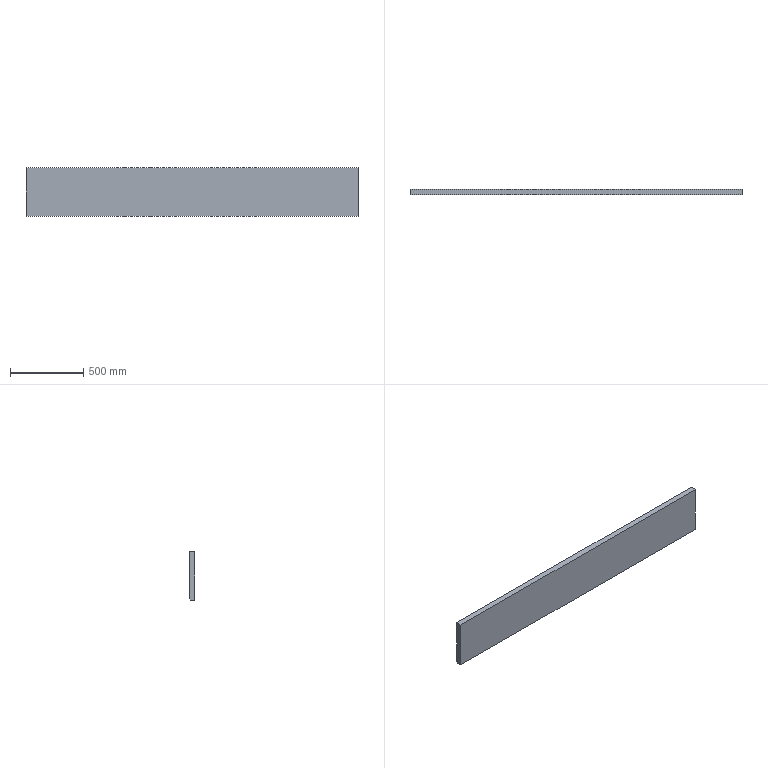Part | SolidWorks | features Chamfer 1, Extrusion 1 | 1 solid | 7 faces | box 2266 x 40 x 333 mm | volume 30069820 mm3 | plane 7
STEP:
#1=CARTESIAN_POINT('',(1133.,30.,-166.5));
#2=VERTEX_POINT('',#1);
#3=CARTESIAN_POINT('',(1133.,0.,-166.5));
#4=VERTEX_POINT('',#3);
#5=CARTESIAN_POINT('',(1133.,40.,-166.5));
#6=DIRECTION('',(0.,-1.,0.));
#7=VECTOR('',#6,1000.);
#8=LINE('',#5,#7);
#9=EDGE_CURVE('',#2,#4,#8,.T.);
#10=ORIENTED_EDGE('',*,*,#9,.F.);
#11=CARTESIAN_POINT('',(1133.,40.,-156.5));
#12=VERTEX_POINT('',#11);
#13=CARTESIAN_POINT('',(1133.,40.,-156.5));
#14=DIRECTION('',(0.,0.7071,0.7071));
#15=VECTOR('',#14,1000.);
#16=LINE('',#13,#15);
#17=EDGE_CURVE('',#2,#12,#16,.T.);
#18=ORIENTED_EDGE('',*,*,#17,.T.);
#19=CARTESIAN_POINT('',(1133.,40.,166.5));
#20=VERTEX_POINT('',#19);
#21=CARTESIAN_POINT('',(1133.,40.,166.5));
#22=DIRECTION('',(0.,0.,-1.));
#23=VECTOR('',#22,1000.);
#24=LINE('',#21,#23);
#25=EDGE_CURVE('',#20,#12,#24,.T.);
#26=ORIENTED_EDGE('',*,*,#25,.F.);
#27=CARTESIAN_POINT('',(1133.,0.,166.5));
#28=VERTEX_POINT('',#27);
#29=CARTESIAN_POINT('',(1133.,40.,166.5));
#30=DIRECTION('',(0.,-1.,0.));
#31=VECTOR('',#30,1000.);
#32=LINE('',#29,#31);
#33=EDGE_CURVE('',#20,#28,#32,.T.);
#34=ORIENTED_EDGE('',*,*,#33,.T.);
#35=CARTESIAN_POINT('',(1133.,0.,166.5));
#36=DIRECTION('',(0.,0.,-1.));
#37=VECTOR('',#36,1000.);
#38=LINE('',#35,#37);
#39=EDGE_CURVE('',#28,#4,#38,.T.);
#40=ORIENTED_EDGE('',*,*,#39,.T.);
#41=EDGE_LOOP('',(#10,#18,#26,#34,#40));
#42=FACE_OUTER_BOUND('',#41,.T.);
#43=CARTESIAN_POINT('',(1133.,40.,166.5));
#44=DIRECTION('',(-1.,0.,0.));
#45=DIRECTION('',(0.,0.,1.));
#46=AXIS2_PLACEMENT_3D('',#43,#44,#45);
#47=PLANE('',#46);
#48=ADVANCED_FACE('',(#42),#47,.F.);
#49=CARTESIAN_POINT('',(-1133.,30.,-166.5));
#50=VERTEX_POINT('',#49);
#51=CARTESIAN_POINT('',(-1133.,0.,-166.5));
#52=VERTEX_POINT('',#51);
#53=CARTESIAN_POINT('',(-1133.,40.,-166.5));
#54=DIRECTION('',(0.,-1.,0.));
#55=VECTOR('',#54,1000.);
#56=LINE('',#53,#55);
#57=EDGE_CURVE('',#50,#52,#56,.T.);
#58=ORIENTED_EDGE('',*,*,#57,.F.);
#59=CARTESIAN_POINT('',(-1133.,30.,-166.5));
#60=DIRECTION('',(1.,0.,0.));
#61=VECTOR('',#60,1000.);
#62=LINE('',#59,#61);
#63=EDGE_CURVE('',#50,#2,#62,.T.);
#64=ORIENTED_EDGE('',*,*,#63,.T.);
#65=ORIENTED_EDGE('',*,*,#9,.T.);
#66=CARTESIAN_POINT('',(-1133.,0.,-166.5));
#67=DIRECTION('',(-1.,0.,0.));
#68=VECTOR('',#67,1000.);
#69=LINE('',#66,#68);
#70=EDGE_CURVE('',#4,#52,#69,.T.);
#71=ORIENTED_EDGE('',*,*,#70,.T.);
#72=EDGE_LOOP('',(#58,#64,#65,#71));
#73=FACE_OUTER_BOUND('',#72,.T.);
#74=CARTESIAN_POINT('',(-1133.,40.,-166.5));
#75=DIRECTION('',(0.,0.,1.));
#76=DIRECTION('',(1.,0.,0.));
#77=AXIS2_PLACEMENT_3D('',#74,#75,#76);
#78=PLANE('',#77);
#79=ADVANCED_FACE('',(#73),#78,.F.);
#80=CARTESIAN_POINT('',(-1133.,40.,-156.5));
#81=VERTEX_POINT('',#80);
#82=CARTESIAN_POINT('',(-1133.,40.,166.5));
#83=VERTEX_POINT('',#82);
#84=CARTESIAN_POINT('',(-1133.,40.,166.5));
#85=DIRECTION('',(0.,0.,1.));
#86=VECTOR('',#85,1000.);
#87=LINE('',#84,#86);
#88=EDGE_CURVE('',#81,#83,#87,.T.);
#89=ORIENTED_EDGE('',*,*,#88,.F.);
#90=CARTESIAN_POINT('',(-1133.,40.,-156.5));
#91=DIRECTION('',(0.,-0.7071,-0.7071));
#92=VECTOR('',#91,1000.);
#93=LINE('',#90,#92);
#94=EDGE_CURVE('',#81,#50,#93,.T.);
#95=ORIENTED_EDGE('',*,*,#94,.T.);
#96=ORIENTED_EDGE('',*,*,#57,.T.);
#97=CARTESIAN_POINT('',(-1133.,0.,166.5));
#98=VERTEX_POINT('',#97);
#99=CARTESIAN_POINT('',(-1133.,0.,166.5));
#100=DIRECTION('',(0.,0.,1.));
#101=VECTOR('',#100,1000.);
#102=LINE('',#99,#101);
#103=EDGE_CURVE('',#52,#98,#102,.T.);
#104=ORIENTED_EDGE('',*,*,#103,.T.);
#105=CARTESIAN_POINT('',(-1133.,40.,166.5));
#106=DIRECTION('',(0.,-1.,0.));
#107=VECTOR('',#106,1000.);
#108=LINE('',#105,#107);
#109=EDGE_CURVE('',#83,#98,#108,.T.);
#110=ORIENTED_EDGE('',*,*,#109,.F.);
#111=EDGE_LOOP('',(#89,#95,#96,#104,#110));
#112=FACE_OUTER_BOUND('',#111,.T.);
#113=CARTESIAN_POINT('',(-1133.,40.,166.5));
#114=DIRECTION('',(1.,0.,0.));
#115=DIRECTION('',(0.,0.,-1.));
#116=AXIS2_PLACEMENT_3D('',#113,#114,#115);
#117=PLANE('',#116);
#118=ADVANCED_FACE('',(#112),#117,.F.);
#119=CARTESIAN_POINT('',(-1133.,0.,166.5));
#120=DIRECTION('',(1.,0.,0.));
#121=VECTOR('',#120,1000.);
#122=LINE('',#119,#121);
#123=EDGE_CURVE('',#98,#28,#122,.T.);
#124=ORIENTED_EDGE('',*,*,#123,.T.);
#125=ORIENTED_EDGE('',*,*,#33,.F.);
#126=CARTESIAN_POINT('',(-1133.,40.,166.5));
#127=DIRECTION('',(1.,0.,0.));
#128=VECTOR('',#127,1000.);
#129=LINE('',#126,#128);
#130=EDGE_CURVE('',#83,#20,#129,.T.);
#131=ORIENTED_EDGE('',*,*,#130,.F.);
#132=ORIENTED_EDGE('',*,*,#109,.T.);
#133=EDGE_LOOP('',(#124,#125,#131,#132));
#134=FACE_OUTER_BOUND('',#133,.T.);
#135=CARTESIAN_POINT('',(-1133.,40.,166.5));
#136=DIRECTION('',(0.,0.,-1.));
#137=DIRECTION('',(-1.,0.,0.));
#138=AXIS2_PLACEMENT_3D('',#135,#136,#137);
#139=PLANE('',#138);
#140=ADVANCED_FACE('',(#134),#139,.F.);
#141=ORIENTED_EDGE('',*,*,#25,.T.);
#142=CARTESIAN_POINT('',(0.,40.,-156.5));
#143=DIRECTION('',(-1.,0.,0.));
#144=VECTOR('',#143,1000.);
#145=LINE('',#142,#144);
#146=EDGE_CURVE('',#12,#81,#145,.T.);
#147=ORIENTED_EDGE('',*,*,#146,.T.);
#148=ORIENTED_EDGE('',*,*,#88,.T.);
#149=ORIENTED_EDGE('',*,*,#130,.T.);
#150=EDGE_LOOP('',(#141,#147,#148,#149));
#151=FACE_OUTER_BOUND('',#150,.T.);
#152=CARTESIAN_POINT('',(0.,40.,0.));
#153=DIRECTION('',(0.,-1.,0.));
#154=DIRECTION('',(0.,0.,-1.));
#155=AXIS2_PLACEMENT_3D('',#152,#153,#154);
#156=PLANE('',#155);
#157=ADVANCED_FACE('',(#151),#156,.F.);
#158=ORIENTED_EDGE('',*,*,#39,.F.);
#159=ORIENTED_EDGE('',*,*,#123,.F.);
#160=ORIENTED_EDGE('',*,*,#103,.F.);
#161=ORIENTED_EDGE('',*,*,#70,.F.);
#162=EDGE_LOOP('',(#158,#159,#160,#161));
#163=FACE_OUTER_BOUND('',#162,.T.);
#164=CARTESIAN_POINT('',(0.,0.,0.));
#165=DIRECTION('',(0.,-1.,0.));
#166=DIRECTION('',(0.,0.,-1.));
#167=AXIS2_PLACEMENT_3D('',#164,#165,#166);
#168=PLANE('',#167);
#169=ADVANCED_FACE('',(#163),#168,.T.);
#170=ORIENTED_EDGE('',*,*,#17,.F.);
#171=ORIENTED_EDGE('',*,*,#63,.F.);
#172=ORIENTED_EDGE('',*,*,#94,.F.);
#173=ORIENTED_EDGE('',*,*,#146,.F.);
#174=EDGE_LOOP('',(#170,#171,#172,#173));
#175=FACE_OUTER_BOUND('',#174,.T.);
#176=CARTESIAN_POINT('',(0.,40.,-156.5));
#177=DIRECTION('',(0.,-0.7071,0.7071));
#178=DIRECTION('',(-1.,0.,0.));
#179=AXIS2_PLACEMENT_3D('',#176,#177,#178);
#180=PLANE('',#179);
#181=ADVANCED_FACE('',(#175),#180,.F.);
#182=CLOSED_SHELL('',(#48,#79,#118,#140,#157,#169,#181));
#183=MANIFOLD_SOLID_BREP('',#182);
#184=CARTESIAN_POINT('',(0.,0.,0.));
#185=DIRECTION('',(0.,0.,1.));
#186=DIRECTION('',(1.,0.,0.));
#187=AXIS2_PLACEMENT_3D('',#184,#185,#186);
#188=(LENGTH_UNIT()NAMED_UNIT(*)SI_UNIT(.MILLI.,.METRE.));
#189=UNCERTAINTY_MEASURE_WITH_UNIT(LENGTH_MEASURE(0.00001),#188,'','');
#190=(NAMED_UNIT(*)PLANE_ANGLE_UNIT()SI_UNIT($,.RADIAN.));
#191=(NAMED_UNIT(*)SI_UNIT($,.STERADIAN.)SOLID_ANGLE_UNIT());
#192=(GEOMETRIC_REPRESENTATION_CONTEXT(3)GLOBAL_UNCERTAINTY_ASSIGNED_CONTEXT((#189))GLOBAL_UNIT_ASSIGNED_CONTEXT((#188,#190,#191))REPRESENTATION_CONTEXT('',''));
#193=ADVANCED_BREP_SHAPE_REPRESENTATION('',(#183,#187),#192);